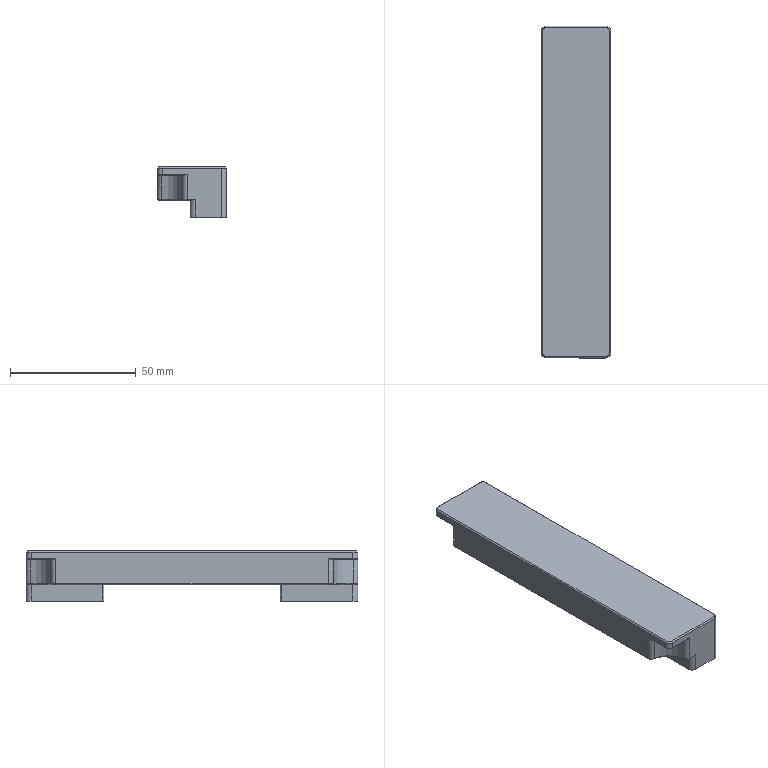NC program | NX | posted with a generic post | part box 27.5 x 132 x 20 mm
Lines 19 to 851 of 2947:
(ZLEVEL_PROFILE_COPY_1 , TOOL : D10)
N36 T15 M6
N38 G54
N40 G17 G0 G90 X-47.703 Y18.85 S9500 M3
N42 G43 Z30. H15
N44 Z1.5
N46 G94 G1 X0. Z-1. F1000.
N48 X64. F3500.
N50 G2 X71.1 Y11.75 R7.1
N52 G1 Y-11.75
N54 G2 X64. Y-18.85 R7.1
N56 G1 X-64.
N58 G2 X-71.1 Y-11.75 R7.1
N60 G1 Y11.75
N62 G2 X-64. Y18.85 R7.1
N64 G1 X0.
N66 X64. Z-1.184
N68 X64.619 Y18.823 Z-1.186
N70 X65.233 Y18.742 Z-1.188
N72 X65.838 Y18.608 Z-1.189
N74 X66.428 Y18.422 Z-1.191
N76 X67.001 Y18.185 Z-1.193
N78 X67.55 Y17.899 Z-1.195
N80 X68.072 Y17.566 Z-1.197
N82 X68.564 Y17.189 Z-1.198
N84 X69.02 Y16.77 Z-1.2
N86 X69.439 Y16.314 Z-1.202
N88 X69.816 Y15.822 Z-1.204
N90 X70.149 Y15.3 Z-1.206
N92 X70.435 Y14.751 Z-1.207
N94 X70.672 Y14.178 Z-1.209
N96 X70.858 Y13.588 Z-1.211
N98 X70.992 Y12.983 Z-1.213
N100 X71.073 Y12.369 Z-1.214
N102 X71.1 Y11.75 Z-1.216
N104 Y-11.75 Z-1.284
N106 X71.073 Y-12.369 Z-1.286
N108 X70.992 Y-12.983 Z-1.287
N110 X70.858 Y-13.588 Z-1.289
N112 X70.672 Y-14.178 Z-1.291
N114 X70.435 Y-14.751 Z-1.293
N116 X70.149 Y-15.3 Z-1.294
N118 X69.816 Y-15.822 Z-1.296
N120 X69.439 Y-16.314 Z-1.298
N122 X69.02 Y-16.77 Z-1.3
N124 X68.564 Y-17.189 Z-1.302
N126 X68.072 Y-17.566 Z-1.303
N128 X67.55 Y-17.899 Z-1.305
N130 X67.001 Y-18.185 Z-1.307
N132 X66.428 Y-18.422 Z-1.309
N134 X65.838 Y-18.608 Z-1.311
N136 X65.233 Y-18.742 Z-1.312
N138 X64.619 Y-18.823 Z-1.314
N140 X64. Y-18.85 Z-1.316
N142 X-54.154 Z-1.656
N144 X-59.077 Z-1.67
N146 X-64. Z-1.684
N148 X-64.619 Y-18.823 Z-1.686
N150 X-65.233 Y-18.742 Z-1.688
N152 X-65.838 Y-18.608 Z-1.689
N154 X-66.428 Y-18.422 Z-1.691
N156 X-67.001 Y-18.185 Z-1.693
N158 X-67.55 Y-17.899 Z-1.695
N160 X-68.072 Y-17.566 Z-1.697
N162 X-68.564 Y-17.189 Z-1.698
N164 X-69.02 Y-16.77 Z-1.7
N166 X-69.439 Y-16.314 Z-1.702
N168 X-69.816 Y-15.822 Z-1.704
N170 X-70.149 Y-15.3 Z-1.706
N172 X-70.435 Y-14.751 Z-1.707
N174 X-70.672 Y-14.178 Z-1.709
N176 X-70.858 Y-13.588 Z-1.711
N178 X-70.992 Y-12.983 Z-1.713
N180 X-71.073 Y-12.369 Z-1.714
N182 X-71.1 Y-11.75 Z-1.716
N184 Y11.75 Z-1.784
N186 X-71.073 Y12.369 Z-1.786
N188 X-70.992 Y12.983 Z-1.787
N190 X-70.858 Y13.588 Z-1.789
N192 X-70.672 Y14.178 Z-1.791
N194 X-70.435 Y14.751 Z-1.793
N196 X-70.149 Y15.3 Z-1.794
N198 X-69.816 Y15.822 Z-1.796
N200 X-69.439 Y16.314 Z-1.798
N202 X-69.02 Y16.77 Z-1.8
N204 X-68.564 Y17.189 Z-1.802
N206 X-68.072 Y17.566 Z-1.803
N208 X-67.55 Y17.899 Z-1.805
N210 X-67.001 Y18.185 Z-1.807
N212 X-66.428 Y18.422 Z-1.809
N214 X-65.838 Y18.608 Z-1.811
N216 X-65.233 Y18.742 Z-1.812
N218 X-64.619 Y18.823 Z-1.814
N220 X-64. Y18.85 Z-1.816
N222 X0. Z-2.
N224 X64. Z-2.184
N226 X64.619 Y18.823 Z-2.186
N228 X65.233 Y18.742 Z-2.188
N230 X65.838 Y18.608 Z-2.189
N232 X66.428 Y18.422 Z-2.191
N234 X67.001 Y18.185 Z-2.193
N236 X67.55 Y17.899 Z-2.195
N238 X68.072 Y17.566 Z-2.197
N240 X68.564 Y17.189 Z-2.198
N242 X69.02 Y16.77 Z-2.2
N244 X69.439 Y16.314 Z-2.202
N246 X69.816 Y15.822 Z-2.204
N248 X70.149 Y15.3 Z-2.206
N250 X70.435 Y14.751 Z-2.207
N252 X70.672 Y14.178 Z-2.209
N254 X70.858 Y13.588 Z-2.211
N256 X70.992 Y12.983 Z-2.213
N258 X71.073 Y12.369 Z-2.214
N260 X71.1 Y11.75 Z-2.216
N262 Y-11.75 Z-2.284
N264 X71.073 Y-12.369 Z-2.286
N266 X70.992 Y-12.983 Z-2.287
N268 X70.858 Y-13.588 Z-2.289
N270 X70.672 Y-14.178 Z-2.291
N272 X70.435 Y-14.751 Z-2.293
N274 X70.149 Y-15.3 Z-2.294
N276 X69.816 Y-15.822 Z-2.296
N278 X69.439 Y-16.314 Z-2.298
N280 X69.02 Y-16.77 Z-2.3
N282 X68.564 Y-17.189 Z-2.302
N284 X68.072 Y-17.566 Z-2.303
N286 X67.55 Y-17.899 Z-2.305
N288 X67.001 Y-18.185 Z-2.307
N290 X66.428 Y-18.422 Z-2.309
N292 X65.838 Y-18.608 Z-2.311
N294 X65.233 Y-18.742 Z-2.312
N296 X64.619 Y-18.823 Z-2.314
N298 X64. Y-18.85 Z-2.316
N300 X-54.154 Z-2.656
N302 X-59.077 Z-2.67
N304 X-64. Z-2.684
N306 X-64.619 Y-18.823 Z-2.686
N308 X-65.233 Y-18.742 Z-2.688
N310 X-65.838 Y-18.608 Z-2.689
N312 X-66.428 Y-18.422 Z-2.691
N314 X-67.001 Y-18.185 Z-2.693
N316 X-67.55 Y-17.899 Z-2.695
N318 X-68.072 Y-17.566 Z-2.697
N320 X-68.564 Y-17.189 Z-2.698
N322 X-69.02 Y-16.77 Z-2.7
N324 X-69.439 Y-16.314 Z-2.702
N326 X-69.816 Y-15.822 Z-2.704
N328 X-70.149 Y-15.3 Z-2.706
N330 X-70.435 Y-14.751 Z-2.707
N332 X-70.672 Y-14.178 Z-2.709
N334 X-70.858 Y-13.588 Z-2.711
N336 X-70.992 Y-12.983 Z-2.713
N338 X-71.073 Y-12.369 Z-2.714
N340 X-71.1 Y-11.75 Z-2.716
N342 Y11.75 Z-2.784
N344 X-71.073 Y12.369 Z-2.786
N346 X-70.992 Y12.983 Z-2.787
N348 X-70.858 Y13.588 Z-2.789
N350 X-70.672 Y14.178 Z-2.791
N352 X-70.435 Y14.751 Z-2.793
N354 X-70.149 Y15.3 Z-2.794
N356 X-69.816 Y15.822 Z-2.796
N358 X-69.439 Y16.314 Z-2.798
N360 X-69.02 Y16.77 Z-2.8
N362 X-68.564 Y17.189 Z-2.802
N364 X-68.072 Y17.566 Z-2.803
N366 X-67.55 Y17.899 Z-2.805
N368 X-67.001 Y18.185 Z-2.807
N370 X-66.428 Y18.422 Z-2.809
N372 X-65.838 Y18.608 Z-2.811
N374 X-65.233 Y18.742 Z-2.812
N376 X-64.619 Y18.823 Z-2.814
N378 X-64. Y18.85 Z-2.816
N380 X0. Z-3.
N382 X64. Z-3.184
N384 X64.619 Y18.823 Z-3.186
N386 X65.233 Y18.742 Z-3.188
N388 X65.838 Y18.608 Z-3.189
N390 X66.428 Y18.422 Z-3.191
N392 X67.001 Y18.185 Z-3.193
N394 X67.55 Y17.899 Z-3.195
N396 X68.072 Y17.566 Z-3.197
N398 X68.564 Y17.189 Z-3.198
N400 X69.02 Y16.77 Z-3.2
N402 X69.439 Y16.314 Z-3.202
N404 X69.816 Y15.822 Z-3.204
N406 X70.149 Y15.3 Z-3.206
N408 X70.435 Y14.751 Z-3.207
N410 X70.672 Y14.178 Z-3.209
N412 X70.858 Y13.588 Z-3.211
N414 X70.992 Y12.983 Z-3.213
N416 X71.073 Y12.369 Z-3.214
N418 X71.1 Y11.75 Z-3.216
N420 Y-11.75 Z-3.284
N422 X71.073 Y-12.369 Z-3.286
N424 X70.992 Y-12.983 Z-3.287
N426 X70.858 Y-13.588 Z-3.289
N428 X70.672 Y-14.178 Z-3.291
N430 X70.435 Y-14.751 Z-3.293
N432 X70.149 Y-15.3 Z-3.294
N434 X69.816 Y-15.822 Z-3.296
N436 X69.439 Y-16.314 Z-3.298
N438 X69.02 Y-16.77 Z-3.3
N440 X68.564 Y-17.189 Z-3.302
N442 X68.072 Y-17.566 Z-3.303
N444 X67.55 Y-17.899 Z-3.305
N446 X67.001 Y-18.185 Z-3.307
N448 X66.428 Y-18.422 Z-3.309
N450 X65.838 Y-18.608 Z-3.311
N452 X65.233 Y-18.742 Z-3.312
N454 X64.619 Y-18.823 Z-3.314
N456 X64. Y-18.85 Z-3.316
N458 X-54.154 Z-3.656
N460 X-59.077 Z-3.67
N462 X-64. Z-3.684
N464 X-64.619 Y-18.823 Z-3.686
N466 X-65.233 Y-18.742 Z-3.688
N468 X-65.838 Y-18.608 Z-3.689
N470 X-66.428 Y-18.422 Z-3.691
N472 X-67.001 Y-18.185 Z-3.693
N474 X-67.55 Y-17.899 Z-3.695
N476 X-68.072 Y-17.566 Z-3.697
N478 X-68.564 Y-17.189 Z-3.698
N480 X-69.02 Y-16.77 Z-3.7
N482 X-69.439 Y-16.314 Z-3.702
N484 X-69.816 Y-15.822 Z-3.704
N486 X-70.149 Y-15.3 Z-3.706
N488 X-70.435 Y-14.751 Z-3.707
N490 X-70.672 Y-14.178 Z-3.709
N492 X-70.858 Y-13.588 Z-3.711
N494 X-70.992 Y-12.983 Z-3.713
N496 X-71.073 Y-12.369 Z-3.714
N498 X-71.1 Y-11.75 Z-3.716
N500 Y11.75 Z-3.784
N502 X-71.073 Y12.369 Z-3.786
N504 X-70.992 Y12.983 Z-3.787
N506 X-70.858 Y13.588 Z-3.789
N508 X-70.672 Y14.178 Z-3.791
N510 X-70.435 Y14.751 Z-3.793
N512 X-70.149 Y15.3 Z-3.794
N514 X-69.816 Y15.822 Z-3.796
N516 X-69.439 Y16.314 Z-3.798
N518 X-69.02 Y16.77 Z-3.8
N520 X-68.564 Y17.189 Z-3.802
N522 X-68.072 Y17.566 Z-3.803
N524 X-67.55 Y17.899 Z-3.805
N526 X-67.001 Y18.185 Z-3.807
N528 X-66.428 Y18.422 Z-3.809
N530 X-65.838 Y18.608 Z-3.811
N532 X-65.233 Y18.742 Z-3.812
N534 X-64.619 Y18.823 Z-3.814
N536 X-64. Y18.85 Z-3.816
N538 X0. Z-4.
N540 X64. Z-4.184
N542 X64.619 Y18.823 Z-4.186
N544 X65.233 Y18.742 Z-4.188
N546 X65.838 Y18.608 Z-4.189
N548 X66.428 Y18.422 Z-4.191
N550 X67.001 Y18.185 Z-4.193
N552 X67.55 Y17.899 Z-4.195
N554 X68.072 Y17.566 Z-4.197
N556 X68.564 Y17.189 Z-4.198
N558 X69.02 Y16.77 Z-4.2
N560 X69.439 Y16.314 Z-4.202
N562 X69.816 Y15.822 Z-4.204
N564 X70.149 Y15.3 Z-4.206
N566 X70.435 Y14.751 Z-4.207
N568 X70.672 Y14.178 Z-4.209
N570 X70.858 Y13.588 Z-4.211
N572 X70.992 Y12.983 Z-4.213
N574 X71.073 Y12.369 Z-4.214
N576 X71.1 Y11.75 Z-4.216
N578 Y-11.75 Z-4.284
N580 X71.073 Y-12.369 Z-4.286
N582 X70.992 Y-12.983 Z-4.287
N584 X70.858 Y-13.588 Z-4.289
N586 X70.672 Y-14.178 Z-4.291
N588 X70.435 Y-14.751 Z-4.293
N590 X70.149 Y-15.3 Z-4.294
N592 X69.816 Y-15.822 Z-4.296
N594 X69.439 Y-16.314 Z-4.298
N596 X69.02 Y-16.77 Z-4.3
N598 X68.564 Y-17.189 Z-4.302
N600 X68.072 Y-17.566 Z-4.303
N602 X67.55 Y-17.899 Z-4.305
N604 X67.001 Y-18.185 Z-4.307
N606 X66.428 Y-18.422 Z-4.309
N608 X65.838 Y-18.608 Z-4.311
N610 X65.233 Y-18.742 Z-4.312
N612 X64.619 Y-18.823 Z-4.314
N614 X64. Y-18.85 Z-4.316
N616 X-54.154 Z-4.656
N618 X-59.077 Z-4.67
N620 X-64. Z-4.684
N622 X-64.619 Y-18.823 Z-4.686
N624 X-65.233 Y-18.742 Z-4.688
N626 X-65.838 Y-18.608 Z-4.689
N628 X-66.428 Y-18.422 Z-4.691
N630 X-67.001 Y-18.185 Z-4.693
N632 X-67.55 Y-17.899 Z-4.695
N634 X-68.072 Y-17.566 Z-4.697
N636 X-68.564 Y-17.189 Z-4.698
N638 X-69.02 Y-16.77 Z-4.7
N640 X-69.439 Y-16.314 Z-4.702
N642 X-69.816 Y-15.822 Z-4.704
N644 X-70.149 Y-15.3 Z-4.706
N646 X-70.435 Y-14.751 Z-4.707
N648 X-70.672 Y-14.178 Z-4.709
N650 X-70.858 Y-13.588 Z-4.711
N652 X-70.992 Y-12.983 Z-4.713
N654 X-71.073 Y-12.369 Z-4.714
N656 X-71.1 Y-11.75 Z-4.716
N658 Y11.75 Z-4.784
N660 X-71.073 Y12.369 Z-4.786
N662 X-70.992 Y12.983 Z-4.787
N664 X-70.858 Y13.588 Z-4.789
N666 X-70.672 Y14.178 Z-4.791
N668 X-70.435 Y14.751 Z-4.793
N670 X-70.149 Y15.3 Z-4.794
N672 X-69.816 Y15.822 Z-4.796
N674 X-69.439 Y16.314 Z-4.798
N676 X-69.02 Y16.77 Z-4.8
N678 X-68.564 Y17.189 Z-4.802
N680 X-68.072 Y17.566 Z-4.803
N682 X-67.55 Y17.899 Z-4.805
N684 X-67.001 Y18.185 Z-4.807
N686 X-66.428 Y18.422 Z-4.809
N688 X-65.838 Y18.608 Z-4.811
N690 X-65.233 Y18.742 Z-4.812
N692 X-64.619 Y18.823 Z-4.814
N694 X-64. Y18.85 Z-4.816
N696 X0. Z-5.
N698 X64. Z-5.184
N700 X64.619 Y18.823 Z-5.186
N702 X65.233 Y18.742 Z-5.188
N704 X65.838 Y18.608 Z-5.189
N706 X66.428 Y18.422 Z-5.191
N708 X67.001 Y18.185 Z-5.193
N710 X67.55 Y17.899 Z-5.195
N712 X68.072 Y17.566 Z-5.197
N714 X68.564 Y17.189 Z-5.198
N716 X69.02 Y16.77 Z-5.2
N718 X69.439 Y16.314 Z-5.202
N720 X69.816 Y15.822 Z-5.204
N722 X70.149 Y15.3 Z-5.206
N724 X70.435 Y14.751 Z-5.207
N726 X70.672 Y14.178 Z-5.209
N728 X70.858 Y13.588 Z-5.211
N730 X70.992 Y12.983 Z-5.213
N732 X71.073 Y12.369 Z-5.214
N734 X71.1 Y11.75 Z-5.216
N736 Y-11.75 Z-5.284
N738 X71.073 Y-12.369 Z-5.286
N740 X70.992 Y-12.983 Z-5.287
N742 X70.858 Y-13.588 Z-5.289
N744 X70.672 Y-14.178 Z-5.291
N746 X70.435 Y-14.751 Z-5.293
N748 X70.149 Y-15.3 Z-5.294
N750 X69.816 Y-15.822 Z-5.296
N752 X69.439 Y-16.314 Z-5.298
N754 X69.02 Y-16.77 Z-5.3
N756 X68.564 Y-17.189 Z-5.302
N758 X68.072 Y-17.566 Z-5.303
N760 X67.55 Y-17.899 Z-5.305
N762 X67.001 Y-18.185 Z-5.307
N764 X66.428 Y-18.422 Z-5.309
N766 X65.838 Y-18.608 Z-5.311
N768 X65.233 Y-18.742 Z-5.312
N770 X64.619 Y-18.823 Z-5.314
N772 X64. Y-18.85 Z-5.316
N774 X-54.154 Z-5.656
N776 X-59.077 Z-5.67
N778 X-64. Z-5.684
N780 X-64.619 Y-18.823 Z-5.686
N782 X-65.233 Y-18.742 Z-5.688
N784 X-65.838 Y-18.608 Z-5.689
N786 X-66.428 Y-18.422 Z-5.691
N788 X-67.001 Y-18.185 Z-5.693
N790 X-67.55 Y-17.899 Z-5.695
N792 X-68.072 Y-17.566 Z-5.697
N794 X-68.564 Y-17.189 Z-5.698
N796 X-69.02 Y-16.77 Z-5.7
N798 X-69.439 Y-16.314 Z-5.702
N800 X-69.816 Y-15.822 Z-5.704
N802 X-70.149 Y-15.3 Z-5.706
N804 X-70.435 Y-14.751 Z-5.707
N806 X-70.672 Y-14.178 Z-5.709
N808 X-70.858 Y-13.588 Z-5.711
N810 X-70.992 Y-12.983 Z-5.713
N812 X-71.073 Y-12.369 Z-5.714
N814 X-71.1 Y-11.75 Z-5.716
N816 Y11.75 Z-5.784
N818 X-71.073 Y12.369 Z-5.786
N820 X-70.992 Y12.983 Z-5.787
N822 X-70.858 Y13.588 Z-5.789
N824 X-70.672 Y14.178 Z-5.791
N826 X-70.435 Y14.751 Z-5.793
N828 X-70.149 Y15.3 Z-5.794
N830 X-69.816 Y15.822 Z-5.796
N832 X-69.439 Y16.314 Z-5.798
N834 X-69.02 Y16.77 Z-5.8
N836 X-68.564 Y17.189 Z-5.802
N838 X-68.072 Y17.566 Z-5.803
N840 X-67.55 Y17.899 Z-5.805
N842 X-67.001 Y18.185 Z-5.807
N844 X-66.428 Y18.422 Z-5.809
N846 X-65.838 Y18.608 Z-5.811
N848 X-65.233 Y18.742 Z-5.812
N850 X-64.619 Y18.823 Z-5.814
N852 X-64. Y18.85 Z-5.816
N854 X0. Z-6.
N856 X64. Z-6.184
N858 X64.619 Y18.823 Z-6.186
N860 X65.233 Y18.742 Z-6.188
N862 X65.838 Y18.608 Z-6.189
N864 X66.428 Y18.422 Z-6.191
N866 X67.001 Y18.185 Z-6.193
N868 X67.55 Y17.899 Z-6.195
N870 X68.072 Y17.566 Z-6.197
N872 X68.564 Y17.189 Z-6.198
N874 X69.02 Y16.77 Z-6.2
N876 X69.439 Y16.314 Z-6.202
N878 X69.816 Y15.822 Z-6.204
N880 X70.149 Y15.3 Z-6.206
N882 X70.435 Y14.751 Z-6.207
N884 X70.672 Y14.178 Z-6.209
N886 X70.858 Y13.588 Z-6.211
N888 X70.992 Y12.983 Z-6.213
N890 X71.073 Y12.369 Z-6.214
N892 X71.1 Y11.75 Z-6.216
N894 Y-11.75 Z-6.284
N896 X71.073 Y-12.369 Z-6.286
N898 X70.992 Y-12.983 Z-6.287
N900 X70.858 Y-13.588 Z-6.289
N902 X70.672 Y-14.178 Z-6.291
N904 X70.435 Y-14.751 Z-6.293
N906 X70.149 Y-15.3 Z-6.294
N908 X69.816 Y-15.822 Z-6.296
N910 X69.439 Y-16.314 Z-6.298
N912 X69.02 Y-16.77 Z-6.3
N914 X68.564 Y-17.189 Z-6.302
N916 X68.072 Y-17.566 Z-6.303
N918 X67.55 Y-17.899 Z-6.305
N920 X67.001 Y-18.185 Z-6.307
N922 X66.428 Y-18.422 Z-6.309
N924 X65.838 Y-18.608 Z-6.311
N926 X65.233 Y-18.742 Z-6.312
N928 X64.619 Y-18.823 Z-6.314
N930 X64. Y-18.85 Z-6.316
N932 X-54.154 Z-6.656
N934 X-59.077 Z-6.67
N936 X-64. Z-6.684
N938 X-64.619 Y-18.823 Z-6.686
N940 X-65.233 Y-18.742 Z-6.688
N942 X-65.838 Y-18.608 Z-6.689
N944 X-66.428 Y-18.422 Z-6.691
N946 X-67.001 Y-18.185 Z-6.693
N948 X-67.55 Y-17.899 Z-6.695
N950 X-68.072 Y-17.566 Z-6.697
N952 X-68.564 Y-17.189 Z-6.698
N954 X-69.02 Y-16.77 Z-6.7
N956 X-69.439 Y-16.314 Z-6.702
N958 X-69.816 Y-15.822 Z-6.704
N960 X-70.149 Y-15.3 Z-6.706
N962 X-70.435 Y-14.751 Z-6.707
N964 X-70.672 Y-14.178 Z-6.709
N966 X-70.858 Y-13.588 Z-6.711
N968 X-70.992 Y-12.983 Z-6.713
N970 X-71.073 Y-12.369 Z-6.714
N972 X-71.1 Y-11.75 Z-6.716
N974 Y11.75 Z-6.784
N976 X-71.073 Y12.369 Z-6.786
N978 X-70.992 Y12.983 Z-6.787
N980 X-70.858 Y13.588 Z-6.789
N982 X-70.672 Y14.178 Z-6.791
N984 X-70.435 Y14.751 Z-6.793
N986 X-70.149 Y15.3 Z-6.794
N988 X-69.816 Y15.822 Z-6.796
N990 X-69.439 Y16.314 Z-6.798
N992 X-69.02 Y16.77 Z-6.8
N994 X-68.564 Y17.189 Z-6.802
N996 X-68.072 Y17.566 Z-6.803
N998 X-67.55 Y17.899 Z-6.805
N1000 X-67.001 Y18.185 Z-6.807
N1002 X-66.428 Y18.422 Z-6.809
N1004 X-65.838 Y18.608 Z-6.811
N1006 X-65.233 Y18.742 Z-6.812
N1008 X-64.619 Y18.823 Z-6.814
N1010 X-64. Y18.85 Z-6.816
N1012 X0. Z-7.
N1014 X64. Z-7.184
N1016 X64.619 Y18.823 Z-7.186
N1018 X65.233 Y18.742 Z-7.188
N1020 X65.838 Y18.608 Z-7.189
N1022 X66.428 Y18.422 Z-7.191
N1024 X67.001 Y18.185 Z-7.193
N1026 X67.55 Y17.899 Z-7.195
N1028 X68.072 Y17.566 Z-7.197
N1030 X68.564 Y17.189 Z-7.198
N1032 X69.02 Y16.77 Z-7.2
N1034 X69.439 Y16.314 Z-7.202
N1036 X69.816 Y15.822 Z-7.204
N1038 X70.149 Y15.3 Z-7.206
N1040 X70.435 Y14.751 Z-7.207
N1042 X70.672 Y14.178 Z-7.209
N1044 X70.858 Y13.588 Z-7.211
N1046 X70.992 Y12.983 Z-7.213
N1048 X71.073 Y12.369 Z-7.214
N1050 X71.1 Y11.75 Z-7.216
N1052 Y-11.75 Z-7.284
N1054 X71.073 Y-12.369 Z-7.286
N1056 X70.992 Y-12.983 Z-7.287
N1058 X70.858 Y-13.588 Z-7.289
N1060 X70.672 Y-14.178 Z-7.291
N1062 X70.435 Y-14.751 Z-7.293
N1064 X70.149 Y-15.3 Z-7.294
N1066 X69.816 Y-15.822 Z-7.296
N1068 X69.439 Y-16.314 Z-7.298
N1070 X69.02 Y-16.77 Z-7.3
N1072 X68.564 Y-17.189 Z-7.302
N1074 X68.072 Y-17.566 Z-7.303
N1076 X67.55 Y-17.899 Z-7.305
N1078 X67.001 Y-18.185 Z-7.307
N1080 X66.428 Y-18.422 Z-7.309
N1082 X65.838 Y-18.608 Z-7.311
N1084 X65.233 Y-18.742 Z-7.312
N1086 X64.619 Y-18.823 Z-7.314
N1088 X64. Y-18.85 Z-7.316
N1090 X-54.154 Z-7.656
N1092 X-59.077 Z-7.67
N1094 X-64. Z-7.684
N1096 X-64.619 Y-18.823 Z-7.686
N1098 X-65.233 Y-18.742 Z-7.688
N1100 X-65.838 Y-18.608 Z-7.689
N1102 X-66.428 Y-18.422 Z-7.691
N1104 X-67.001 Y-18.185 Z-7.693
N1106 X-67.55 Y-17.899 Z-7.695
N1108 X-68.072 Y-17.566 Z-7.697
N1110 X-68.564 Y-17.189 Z-7.698
N1112 X-69.02 Y-16.77 Z-7.7
N1114 X-69.439 Y-16.314 Z-7.702
N1116 X-69.816 Y-15.822 Z-7.704
N1118 X-70.149 Y-15.3 Z-7.706
N1120 X-70.435 Y-14.751 Z-7.707
N1122 X-70.672 Y-14.178 Z-7.709
N1124 X-70.858 Y-13.588 Z-7.711
N1126 X-70.992 Y-12.983 Z-7.713
N1128 X-71.073 Y-12.369 Z-7.714
N1130 X-71.1 Y-11.75 Z-7.716
N1132 Y11.75 Z-7.784
N1134 X-71.073 Y12.369 Z-7.786
N1136 X-70.992 Y12.983 Z-7.787
N1138 X-70.858 Y13.588 Z-7.789
N1140 X-70.672 Y14.178 Z-7.791
N1142 X-70.435 Y14.751 Z-7.793
N1144 X-70.149 Y15.3 Z-7.794
N1146 X-69.816 Y15.822 Z-7.796
N1148 X-69.439 Y16.314 Z-7.798
N1150 X-69.02 Y16.77 Z-7.8
N1152 X-68.564 Y17.189 Z-7.802
N1154 X-68.072 Y17.566 Z-7.803
N1156 X-67.55 Y17.899 Z-7.805
N1158 X-67.001 Y18.185 Z-7.807
N1160 X-66.428 Y18.422 Z-7.809
N1162 X-65.838 Y18.608 Z-7.811
N1164 X-65.233 Y18.742 Z-7.812
N1166 X-64.619 Y18.823 Z-7.814
N1168 X-64. Y18.85 Z-7.816
N1170 X0. Z-8.
N1172 X64. Z-8.184
N1174 X64.619 Y18.823 Z-8.186
N1176 X65.233 Y18.742 Z-8.188
N1178 X65.838 Y18.608 Z-8.189
N1180 X66.428 Y18.422 Z-8.191
N1182 X67.001 Y18.185 Z-8.193
N1184 X67.55 Y17.899 Z-8.195
N1186 X68.072 Y17.566 Z-8.197
N1188 X68.564 Y17.189 Z-8.198
N1190 X69.02 Y16.77 Z-8.2
N1192 X69.439 Y16.314 Z-8.202
N1194 X69.816 Y15.822 Z-8.204
N1196 X70.149 Y15.3 Z-8.206
N1198 X70.435 Y14.751 Z-8.207
N1200 X70.672 Y14.178 Z-8.209
N1202 X70.858 Y13.588 Z-8.211
N1204 X70.992 Y12.983 Z-8.213
N1206 X71.073 Y12.369 Z-8.214
N1208 X71.1 Y11.75 Z-8.216
N1210 Y-11.75 Z-8.284
N1212 X71.073 Y-12.369 Z-8.286
N1214 X70.992 Y-12.983 Z-8.287
N1216 X70.858 Y-13.588 Z-8.289
N1218 X70.672 Y-14.178 Z-8.291
N1220 X70.435 Y-14.751 Z-8.293
N1222 X70.149 Y-15.3 Z-8.294
N1224 X69.816 Y-15.822 Z-8.296
N1226 X69.439 Y-16.314 Z-8.298
N1228 X69.02 Y-16.77 Z-8.3
N1230 X68.564 Y-17.189 Z-8.302
N1232 X68.072 Y-17.566 Z-8.303
N1234 X67.55 Y-17.899 Z-8.305
N1236 X67.001 Y-18.185 Z-8.307
N1238 X66.428 Y-18.422 Z-8.309
N1240 X65.838 Y-18.608 Z-8.311
N1242 X65.233 Y-18.742 Z-8.312
N1244 X64.619 Y-18.823 Z-8.314
N1246 X64. Y-18.85 Z-8.316
N1248 X-54.154 Z-8.656
N1250 X-59.077 Z-8.67
N1252 X-64. Z-8.684
N1254 X-64.619 Y-18.823 Z-8.686
N1256 X-65.233 Y-18.742 Z-8.688
N1258 X-65.838 Y-18.608 Z-8.689
N1260 X-66.428 Y-18.422 Z-8.691
N1262 X-67.001 Y-18.185 Z-8.693
N1264 X-67.55 Y-17.899 Z-8.695
N1266 X-68.072 Y-17.566 Z-8.697
N1268 X-68.564 Y-17.189 Z-8.698
N1270 X-69.02 Y-16.77 Z-8.7
N1272 X-69.439 Y-16.314 Z-8.702
N1274 X-69.816 Y-15.822 Z-8.704
N1276 X-70.149 Y-15.3 Z-8.706
N1278 X-70.435 Y-14.751 Z-8.707
N1280 X-70.672 Y-14.178 Z-8.709
N1282 X-70.858 Y-13.588 Z-8.711
N1284 X-70.992 Y-12.983 Z-8.713
N1286 X-71.073 Y-12.369 Z-8.714
N1288 X-71.1 Y-11.75 Z-8.716
N1290 Y11.75 Z-8.784
N1292 X-71.073 Y12.369 Z-8.786
N1294 X-70.992 Y12.983 Z-8.787
N1296 X-70.858 Y13.588 Z-8.789
N1298 X-70.672 Y14.178 Z-8.791
N1300 X-70.435 Y14.751 Z-8.793
N1302 X-70.149 Y15.3 Z-8.794
N1304 X-69.816 Y15.822 Z-8.796
N1306 X-69.439 Y16.314 Z-8.798
N1308 X-69.02 Y16.77 Z-8.8
N1310 X-68.564 Y17.189 Z-8.802
N1312 X-68.072 Y17.566 Z-8.803
N1314 X-67.55 Y17.899 Z-8.805
N1316 X-67.001 Y18.185 Z-8.807
N1318 X-66.428 Y18.422 Z-8.809
N1320 X-65.838 Y18.608 Z-8.811
N1322 X-65.233 Y18.742 Z-8.812
N1324 X-64.619 Y18.823 Z-8.814
N1326 X-64. Y18.85 Z-8.816
N1328 X0. Z-9.
N1330 X64. Z-9.184
N1332 X64.619 Y18.823 Z-9.186
N1334 X65.233 Y18.742 Z-9.188
N1336 X65.838 Y18.608 Z-9.189
N1338 X66.428 Y18.422 Z-9.191
N1340 X67.001 Y18.185 Z-9.193
N1342 X67.55 Y17.899 Z-9.195
N1344 X68.072 Y17.566 Z-9.197
N1346 X68.564 Y17.189 Z-9.198
N1348 X69.02 Y16.77 Z-9.2
N1350 X69.439 Y16.314 Z-9.202
N1352 X69.816 Y15.822 Z-9.204
N1354 X70.149 Y15.3 Z-9.206
N1356 X70.435 Y14.751 Z-9.207
N1358 X70.672 Y14.178 Z-9.209
N1360 X70.858 Y13.588 Z-9.211
N1362 X70.992 Y12.983 Z-9.213
N1364 X71.073 Y12.369 Z-9.214
N1366 X71.1 Y11.75 Z-9.216
N1368 Y-11.75 Z-9.284
N1370 X71.073 Y-12.369 Z-9.286
N1372 X70.992 Y-12.983 Z-9.287
N1374 X70.858 Y-13.588 Z-9.289
N1376 X70.672 Y-14.178 Z-9.291
N1378 X70.435 Y-14.751 Z-9.293
N1380 X70.149 Y-15.3 Z-9.294
N1382 X69.816 Y-15.822 Z-9.296
N1384 X69.439 Y-16.314 Z-9.298
N1386 X69.02 Y-16.77 Z-9.3
N1388 X68.564 Y-17.189 Z-9.302
N1390 X68.072 Y-17.566 Z-9.303
N1392 X67.55 Y-17.899 Z-9.305
N1394 X67.001 Y-18.185 Z-9.307
N1396 X66.428 Y-18.422 Z-9.309
N1398 X65.838 Y-18.608 Z-9.311
N1400 X65.233 Y-18.742 Z-9.312
N1402 X64.619 Y-18.823 Z-9.314
N1404 X64. Y-18.85 Z-9.316
N1406 X-54.154 Z-9.656
N1408 X-59.077 Z-9.67
N1410 X-64. Z-9.684
N1412 X-64.619 Y-18.823 Z-9.686
N1414 X-65.233 Y-18.742 Z-9.688
N1416 X-65.838 Y-18.608 Z-9.689
N1418 X-66.428 Y-18.422 Z-9.691
N1420 X-67.001 Y-18.185 Z-9.693
N1422 X-67.55 Y-17.899 Z-9.695
N1424 X-68.072 Y-17.566 Z-9.697
N1426 X-68.564 Y-17.189 Z-9.698
N1428 X-69.02 Y-16.77 Z-9.7
N1430 X-69.439 Y-16.314 Z-9.702
N1432 X-69.816 Y-15.822 Z-9.704
N1434 X-70.149 Y-15.3 Z-9.706
N1436 X-70.435 Y-14.751 Z-9.707
N1438 X-70.672 Y-14.178 Z-9.709
N1440 X-70.858 Y-13.588 Z-9.711
N1442 X-70.992 Y-12.983 Z-9.713
N1444 X-71.073 Y-12.369 Z-9.714
N1446 X-71.1 Y-11.75 Z-9.716
N1448 Y11.75 Z-9.784
N1450 X-71.073 Y12.369 Z-9.786
N1452 X-70.992 Y12.983 Z-9.787
N1454 X-70.858 Y13.588 Z-9.789
N1456 X-70.672 Y14.178 Z-9.791
N1458 X-70.435 Y14.751 Z-9.793
N1460 X-70.149 Y15.3 Z-9.794
N1462 X-69.816 Y15.822 Z-9.796
N1464 X-69.439 Y16.314 Z-9.798
N1466 X-69.02 Y16.77 Z-9.8
N1468 X-68.564 Y17.189 Z-9.802
N1470 X-68.072 Y17.566 Z-9.803
N1472 X-67.55 Y17.899 Z-9.805
N1474 X-67.001 Y18.185 Z-9.807
N1476 X-66.428 Y18.422 Z-9.809
N1478 X-65.838 Y18.608 Z-9.811
N1480 X-65.233 Y18.742 Z-9.812
N1482 X-64.619 Y18.823 Z-9.814
N1484 X-64. Y18.85 Z-9.816
N1486 X0. Z-10.
N1488 X64. Z-10.184
N1490 X64.619 Y18.823 Z-10.186
N1492 X65.233 Y18.742 Z-10.188
N1494 X65.838 Y18.608 Z-10.189
N1496 X66.428 Y18.422 Z-10.191
N1498 X67.001 Y18.185 Z-10.193
N1500 X67.55 Y17.899 Z-10.195
N1502 X68.072 Y17.566 Z-10.197
N1504 X68.564 Y17.189 Z-10.198
N1506 X69.02 Y16.77 Z-10.2
N1508 X69.439 Y16.314 Z-10.202
N1510 X69.816 Y15.822 Z-10.204
N1512 X70.149 Y15.3 Z-10.206
N1514 X70.435 Y14.751 Z-10.207
N1516 X70.672 Y14.178 Z-10.209
N1518 X70.858 Y13.588 Z-10.211
N1520 X70.992 Y12.983 Z-10.213
N1522 X71.073 Y12.369 Z-10.214
N1524 X71.1 Y11.75 Z-10.216
N1526 Y-11.75 Z-10.284
N1528 X71.073 Y-12.369 Z-10.286
N1530 X70.992 Y-12.983 Z-10.287
N1532 X70.858 Y-13.588 Z-10.289
N1534 X70.672 Y-14.178 Z-10.291
N1536 X70.435 Y-14.751 Z-10.293
N1538 X70.149 Y-15.3 Z-10.294
N1540 X69.816 Y-15.822 Z-10.296
N1542 X69.439 Y-16.314 Z-10.298
N1544 X69.02 Y-16.77 Z-10.3
N1546 X68.564 Y-17.189 Z-10.302
N1548 X68.072 Y-17.566 Z-10.303
N1550 X67.55 Y-17.899 Z-10.305
N1552 X67.001 Y-18.185 Z-10.307
N1554 X66.428 Y-18.422 Z-10.309
N1556 X65.838 Y-18.608 Z-10.311
N1558 X65.233 Y-18.742 Z-10.312
N1560 X64.619 Y-18.823 Z-10.314
N1562 X64. Y-18.85 Z-10.316
N1564 X-54.154 Z-10.656
N1566 X-59.077 Z-10.67
N1568 X-64. Z-10.684
N1570 X-64.619 Y-18.823 Z-10.686
N1572 X-65.233 Y-18.742 Z-10.688
N1574 X-65.838 Y-18.608 Z-10.689
N1576 X-66.428 Y-18.422 Z-10.691
N1578 X-67.001 Y-18.185 Z-10.693
N1580 X-67.55 Y-17.899 Z-10.695
N1582 X-68.072 Y-17.566 Z-10.697
N1584 X-68.564 Y-17.189 Z-10.698
N1586 X-69.02 Y-16.77 Z-10.7
N1588 X-69.439 Y-16.314 Z-10.702
N1590 X-69.816 Y-15.822 Z-10.704
N1592 X-70.149 Y-15.3 Z-10.706
N1594 X-70.435 Y-14.751 Z-10.707
N1596 X-70.672 Y-14.178 Z-10.709
N1598 X-70.858 Y-13.588 Z-10.711
N1600 X-70.992 Y-12.983 Z-10.713
N1602 X-71.073 Y-12.369 Z-10.714
N1604 X-71.1 Y-11.75 Z-10.716
N1606 Y11.75 Z-10.784
N1608 X-71.073 Y12.369 Z-10.786
N1610 X-70.992 Y12.983 Z-10.787
N1612 X-70.858 Y13.588 Z-10.789
N1614 X-70.672 Y14.178 Z-10.791
N1616 X-70.435 Y14.751 Z-10.793
N1618 X-70.149 Y15.3 Z-10.794
N1620 X-69.816 Y15.822 Z-10.796
N1622 X-69.439 Y16.314 Z-10.798
N1624 X-69.02 Y16.77 Z-10.8
N1626 X-68.564 Y17.189 Z-10.802
N1628 X-68.072 Y17.566 Z-10.803
N1630 X-67.55 Y17.899 Z-10.805
N1632 X-67.001 Y18.185 Z-10.807
N1634 X-66.428 Y18.422 Z-10.809
N1636 X-65.838 Y18.608 Z-10.811
N1638 X-65.233 Y18.742 Z-10.812
N1640 X-64.619 Y18.823 Z-10.814
N1642 X-64. Y18.85 Z-10.816
N1644 X0. Z-11.
N1646 X64. Z-11.184
N1648 X64.619 Y18.823 Z-11.186
N1650 X65.233 Y18.742 Z-11.188
N1652 X65.838 Y18.608 Z-11.189
N1654 X66.428 Y18.422 Z-11.191
N1656 X67.001 Y18.185 Z-11.193
N1658 X67.55 Y17.899 Z-11.195
N1660 X68.072 Y17.566 Z-11.197
N1662 X68.564 Y17.189 Z-11.198
N1664 X69.02 Y16.77 Z-11.2
N1666 X69.439 Y16.314 Z-11.202
N1668 X69.816 Y15.822 Z-11.204
N1670 X70.149 Y15.3 Z-11.206
N1672 X70.435 Y14.751 Z-11.207
N1674 X70.672 Y14.178 Z-11.209
N1676 X70.858 Y13.588 Z-11.211
N1678 X70.992 Y12.983 Z-11.213
N1680 X71.073 Y12.369 Z-11.214
N1682 X71.1 Y11.75 Z-11.216
N1684 Y-11.75 Z-11.284
N1686 X71.073 Y-12.369 Z-11.286
N1688 X70.992 Y-12.983 Z-11.287
N1690 X70.858 Y-13.588 Z-11.289
N1692 X70.672 Y-14.178 Z-11.291
N1694 X70.435 Y-14.751 Z-11.293